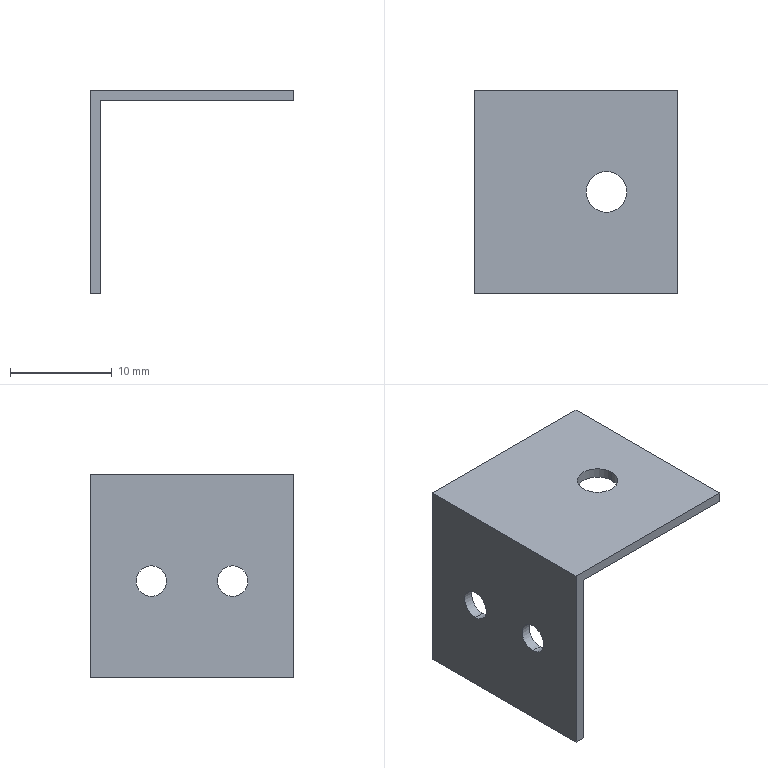Part | SolidWorks | features BaseBody 1 | 1 solid | 14 faces | box 20 x 20 x 20 mm | volume 753.296 mm3 | plane 8 | cylinder 6 | commonest cylinder face diameters 3 x4 4 x2
STEP:
#1=CARTESIAN_POINT('',(1.,10.,10.));
#2=VERTEX_POINT('',#1);
#3=CARTESIAN_POINT('',(5.,10.,10.));
#4=VERTEX_POINT('',#3);
#5=CARTESIAN_POINT('',(3.,10.,10.));
#6=DIRECTION('',(0.,0.,1.));
#7=DIRECTION('',(-1.,0.,0.));
#8=AXIS2_PLACEMENT_3D('',#5,#6,#7);
#9=CIRCLE('',#8,2.);
#10=EDGE_CURVE('',#2,#4,#9,.T.);
#11=ORIENTED_EDGE('',*,*,#10,.T.);
#12=CARTESIAN_POINT('',(5.,10.,9.));
#13=VERTEX_POINT('',#12);
#14=CARTESIAN_POINT('',(5.,10.,10.));
#15=DIRECTION('',(0.,0.,-1.));
#16=VECTOR('',#15,1000.);
#17=LINE('',#14,#16);
#18=EDGE_CURVE('',#4,#13,#17,.T.);
#19=ORIENTED_EDGE('',*,*,#18,.T.);
#20=CARTESIAN_POINT('',(1.,10.,9.));
#21=VERTEX_POINT('',#20);
#22=CARTESIAN_POINT('',(3.,10.,9.));
#23=DIRECTION('',(0.,0.,1.));
#24=DIRECTION('',(-1.,0.,0.));
#25=AXIS2_PLACEMENT_3D('',#22,#23,#24);
#26=CIRCLE('',#25,2.);
#27=EDGE_CURVE('',#21,#13,#26,.T.);
#28=ORIENTED_EDGE('',*,*,#27,.F.);
#29=CARTESIAN_POINT('',(1.,10.,10.));
#30=DIRECTION('',(0.,0.,-1.));
#31=VECTOR('',#30,1000.);
#32=LINE('',#29,#31);
#33=EDGE_CURVE('',#2,#21,#32,.T.);
#34=ORIENTED_EDGE('',*,*,#33,.F.);
#35=EDGE_LOOP('',(#11,#19,#28,#34));
#36=FACE_OUTER_BOUND('',#35,.T.);
#37=CARTESIAN_POINT('',(3.,10.,10.));
#38=DIRECTION('',(0.,0.,-1.));
#39=DIRECTION('',(-1.,0.,0.));
#40=AXIS2_PLACEMENT_3D('',#37,#38,#39);
#41=CYLINDRICAL_SURFACE('',#40,2.);
#42=ADVANCED_FACE('',(#36),#41,.F.);
#43=CARTESIAN_POINT('',(-10.,6.,1.));
#44=VERTEX_POINT('',#43);
#45=CARTESIAN_POINT('',(-10.,6.,-2.));
#46=VERTEX_POINT('',#45);
#47=CARTESIAN_POINT('',(-10.,6.,-0.5));
#48=DIRECTION('',(1.,0.,0.));
#49=DIRECTION('',(0.,0.,-1.));
#50=AXIS2_PLACEMENT_3D('',#47,#48,#49);
#51=CIRCLE('',#50,1.5);
#52=EDGE_CURVE('',#44,#46,#51,.T.);
#53=ORIENTED_EDGE('',*,*,#52,.F.);
#54=CARTESIAN_POINT('',(-9.,6.,1.));
#55=VERTEX_POINT('',#54);
#56=CARTESIAN_POINT('',(-29.,6.,1.));
#57=DIRECTION('',(1.,0.,0.));
#58=VECTOR('',#57,1000.);
#59=LINE('',#56,#58);
#60=EDGE_CURVE('',#44,#55,#59,.T.);
#61=ORIENTED_EDGE('',*,*,#60,.T.);
#62=CARTESIAN_POINT('',(-9.,6.,-2.));
#63=VERTEX_POINT('',#62);
#64=CARTESIAN_POINT('',(-9.,6.,-0.5));
#65=DIRECTION('',(-1.,0.,0.));
#66=DIRECTION('',(0.,0.,-1.));
#67=AXIS2_PLACEMENT_3D('',#64,#65,#66);
#68=CIRCLE('',#67,1.5);
#69=EDGE_CURVE('',#63,#55,#68,.T.);
#70=ORIENTED_EDGE('',*,*,#69,.F.);
#71=CARTESIAN_POINT('',(-29.,6.,-2.));
#72=DIRECTION('',(1.,0.,0.));
#73=VECTOR('',#72,1000.);
#74=LINE('',#71,#73);
#75=EDGE_CURVE('',#46,#63,#74,.T.);
#76=ORIENTED_EDGE('',*,*,#75,.F.);
#77=EDGE_LOOP('',(#53,#61,#70,#76));
#78=FACE_OUTER_BOUND('',#77,.T.);
#79=CARTESIAN_POINT('',(-29.,6.,-0.5));
#80=DIRECTION('',(1.,0.,0.));
#81=DIRECTION('',(0.,0.,-1.));
#82=AXIS2_PLACEMENT_3D('',#79,#80,#81);
#83=CYLINDRICAL_SURFACE('',#82,1.5);
#84=ADVANCED_FACE('',(#78),#83,.F.);
#85=CARTESIAN_POINT('',(-10.,14.,1.));
#86=VERTEX_POINT('',#85);
#87=CARTESIAN_POINT('',(-10.,14.,-2.));
#88=VERTEX_POINT('',#87);
#89=CARTESIAN_POINT('',(-10.,14.,-0.5));
#90=DIRECTION('',(1.,0.,0.));
#91=DIRECTION('',(0.,0.,-1.));
#92=AXIS2_PLACEMENT_3D('',#89,#90,#91);
#93=CIRCLE('',#92,1.5);
#94=EDGE_CURVE('',#86,#88,#93,.T.);
#95=ORIENTED_EDGE('',*,*,#94,.F.);
#96=CARTESIAN_POINT('',(-9.,14.,1.));
#97=VERTEX_POINT('',#96);
#98=CARTESIAN_POINT('',(-29.,14.,1.));
#99=DIRECTION('',(1.,0.,0.));
#100=VECTOR('',#99,1000.);
#101=LINE('',#98,#100);
#102=EDGE_CURVE('',#86,#97,#101,.T.);
#103=ORIENTED_EDGE('',*,*,#102,.T.);
#104=CARTESIAN_POINT('',(-9.,14.,-2.));
#105=VERTEX_POINT('',#104);
#106=CARTESIAN_POINT('',(-9.,14.,-0.5));
#107=DIRECTION('',(-1.,0.,0.));
#108=DIRECTION('',(0.,0.,-1.));
#109=AXIS2_PLACEMENT_3D('',#106,#107,#108);
#110=CIRCLE('',#109,1.5);
#111=EDGE_CURVE('',#105,#97,#110,.T.);
#112=ORIENTED_EDGE('',*,*,#111,.F.);
#113=CARTESIAN_POINT('',(-29.,14.,-2.));
#114=DIRECTION('',(1.,0.,0.));
#115=VECTOR('',#114,1000.);
#116=LINE('',#113,#115);
#117=EDGE_CURVE('',#88,#105,#116,.T.);
#118=ORIENTED_EDGE('',*,*,#117,.F.);
#119=EDGE_LOOP('',(#95,#103,#112,#118));
#120=FACE_OUTER_BOUND('',#119,.T.);
#121=CARTESIAN_POINT('',(-29.,14.,-0.5));
#122=DIRECTION('',(1.,0.,0.));
#123=DIRECTION('',(0.,0.,-1.));
#124=AXIS2_PLACEMENT_3D('',#121,#122,#123);
#125=CYLINDRICAL_SURFACE('',#124,1.5);
#126=ADVANCED_FACE('',(#120),#125,.F.);
#127=CARTESIAN_POINT('',(10.,20.,10.));
#128=VERTEX_POINT('',#127);
#129=CARTESIAN_POINT('',(10.,0.,10.));
#130=VERTEX_POINT('',#129);
#131=CARTESIAN_POINT('',(10.,20.,10.));
#132=DIRECTION('',(0.,-1.,0.));
#133=VECTOR('',#132,1000.);
#134=LINE('',#131,#133);
#135=EDGE_CURVE('',#128,#130,#134,.T.);
#136=ORIENTED_EDGE('',*,*,#135,.F.);
#137=CARTESIAN_POINT('',(-10.,20.,10.));
#138=VERTEX_POINT('',#137);
#139=CARTESIAN_POINT('',(0.,20.,10.));
#140=DIRECTION('',(1.,0.,0.));
#141=VECTOR('',#140,1000.);
#142=LINE('',#139,#141);
#143=EDGE_CURVE('',#138,#128,#142,.T.);
#144=ORIENTED_EDGE('',*,*,#143,.F.);
#145=CARTESIAN_POINT('',(-10.,0.,10.));
#146=VERTEX_POINT('',#145);
#147=CARTESIAN_POINT('',(-10.,20.,10.));
#148=DIRECTION('',(0.,1.,0.));
#149=VECTOR('',#148,1000.);
#150=LINE('',#147,#149);
#151=EDGE_CURVE('',#146,#138,#150,.T.);
#152=ORIENTED_EDGE('',*,*,#151,.F.);
#153=CARTESIAN_POINT('',(0.,0.,10.));
#154=DIRECTION('',(-1.,0.,0.));
#155=VECTOR('',#154,1000.);
#156=LINE('',#153,#155);
#157=EDGE_CURVE('',#130,#146,#156,.T.);
#158=ORIENTED_EDGE('',*,*,#157,.F.);
#159=EDGE_LOOP('',(#136,#144,#152,#158));
#160=FACE_OUTER_BOUND('',#159,.T.);
#161=ORIENTED_EDGE('',*,*,#10,.F.);
#162=CARTESIAN_POINT('',(3.,10.,10.));
#163=DIRECTION('',(0.,0.,1.));
#164=DIRECTION('',(-1.,0.,0.));
#165=AXIS2_PLACEMENT_3D('',#162,#163,#164);
#166=CIRCLE('',#165,2.);
#167=EDGE_CURVE('',#4,#2,#166,.T.);
#168=ORIENTED_EDGE('',*,*,#167,.F.);
#169=EDGE_LOOP('',(#161,#168));
#170=FACE_BOUND('',#169,.T.);
#171=CARTESIAN_POINT('',(0.,20.,10.));
#172=DIRECTION('',(0.,0.,-1.));
#173=DIRECTION('',(-1.,0.,0.));
#174=AXIS2_PLACEMENT_3D('',#171,#172,#173);
#175=PLANE('',#174);
#176=ADVANCED_FACE('',(#160,#170),#175,.F.);
#177=CARTESIAN_POINT('',(10.,0.,9.));
#178=VERTEX_POINT('',#177);
#179=CARTESIAN_POINT('',(-9.,0.,9.));
#180=VERTEX_POINT('',#179);
#181=CARTESIAN_POINT('',(0.,0.,9.));
#182=DIRECTION('',(-1.,0.,0.));
#183=VECTOR('',#182,1000.);
#184=LINE('',#181,#183);
#185=EDGE_CURVE('',#178,#180,#184,.T.);
#186=ORIENTED_EDGE('',*,*,#185,.F.);
#187=CARTESIAN_POINT('',(10.,0.,0.));
#188=DIRECTION('',(0.,0.,-1.));
#189=VECTOR('',#188,1000.);
#190=LINE('',#187,#189);
#191=EDGE_CURVE('',#130,#178,#190,.T.);
#192=ORIENTED_EDGE('',*,*,#191,.F.);
#193=ORIENTED_EDGE('',*,*,#157,.T.);
#194=CARTESIAN_POINT('',(-10.,0.,-10.));
#195=VERTEX_POINT('',#194);
#196=CARTESIAN_POINT('',(-10.,0.,0.));
#197=DIRECTION('',(0.,0.,1.));
#198=VECTOR('',#197,1000.);
#199=LINE('',#196,#198);
#200=EDGE_CURVE('',#195,#146,#199,.T.);
#201=ORIENTED_EDGE('',*,*,#200,.F.);
#202=CARTESIAN_POINT('',(-9.,0.,-10.));
#203=VERTEX_POINT('',#202);
#204=CARTESIAN_POINT('',(0.,0.,-10.));
#205=DIRECTION('',(-1.,0.,0.));
#206=VECTOR('',#205,1000.);
#207=LINE('',#204,#206);
#208=EDGE_CURVE('',#203,#195,#207,.T.);
#209=ORIENTED_EDGE('',*,*,#208,.F.);
#210=CARTESIAN_POINT('',(-9.,0.,0.));
#211=DIRECTION('',(0.,0.,-1.));
#212=VECTOR('',#211,1000.);
#213=LINE('',#210,#212);
#214=EDGE_CURVE('',#180,#203,#213,.T.);
#215=ORIENTED_EDGE('',*,*,#214,.F.);
#216=EDGE_LOOP('',(#186,#192,#193,#201,#209,#215));
#217=FACE_OUTER_BOUND('',#216,.T.);
#218=CARTESIAN_POINT('',(0.,0.,0.));
#219=DIRECTION('',(0.,1.,0.));
#220=DIRECTION('',(0.,0.,1.));
#221=AXIS2_PLACEMENT_3D('',#218,#219,#220);
#222=PLANE('',#221);
#223=ADVANCED_FACE('',(#217),#222,.F.);
#224=CARTESIAN_POINT('',(10.,20.,9.));
#225=VERTEX_POINT('',#224);
#226=CARTESIAN_POINT('',(10.,20.,9.));
#227=DIRECTION('',(0.,-1.,0.));
#228=VECTOR('',#227,1000.);
#229=LINE('',#226,#228);
#230=EDGE_CURVE('',#225,#178,#229,.T.);
#231=ORIENTED_EDGE('',*,*,#230,.F.);
#232=CARTESIAN_POINT('',(10.,20.,0.));
#233=DIRECTION('',(0.,0.,-1.));
#234=VECTOR('',#233,1000.);
#235=LINE('',#232,#234);
#236=EDGE_CURVE('',#128,#225,#235,.T.);
#237=ORIENTED_EDGE('',*,*,#236,.F.);
#238=ORIENTED_EDGE('',*,*,#135,.T.);
#239=ORIENTED_EDGE('',*,*,#191,.T.);
#240=EDGE_LOOP('',(#231,#237,#238,#239));
#241=FACE_OUTER_BOUND('',#240,.T.);
#242=CARTESIAN_POINT('',(10.,20.,0.));
#243=DIRECTION('',(-1.,0.,0.));
#244=DIRECTION('',(0.,0.,1.));
#245=AXIS2_PLACEMENT_3D('',#242,#243,#244);
#246=PLANE('',#245);
#247=ADVANCED_FACE('',(#241),#246,.F.);
#248=ORIENTED_EDGE('',*,*,#236,.T.);
#249=CARTESIAN_POINT('',(-9.,20.,9.));
#250=VERTEX_POINT('',#249);
#251=CARTESIAN_POINT('',(0.,20.,9.));
#252=DIRECTION('',(-1.,0.,0.));
#253=VECTOR('',#252,1000.);
#254=LINE('',#251,#253);
#255=EDGE_CURVE('',#225,#250,#254,.T.);
#256=ORIENTED_EDGE('',*,*,#255,.T.);
#257=CARTESIAN_POINT('',(-9.,20.,-10.));
#258=VERTEX_POINT('',#257);
#259=CARTESIAN_POINT('',(-9.,20.,0.));
#260=DIRECTION('',(0.,0.,-1.));
#261=VECTOR('',#260,1000.);
#262=LINE('',#259,#261);
#263=EDGE_CURVE('',#250,#258,#262,.T.);
#264=ORIENTED_EDGE('',*,*,#263,.T.);
#265=CARTESIAN_POINT('',(-10.,20.,-10.));
#266=VERTEX_POINT('',#265);
#267=CARTESIAN_POINT('',(0.,20.,-10.));
#268=DIRECTION('',(1.,0.,0.));
#269=VECTOR('',#268,1000.);
#270=LINE('',#267,#269);
#271=EDGE_CURVE('',#266,#258,#270,.T.);
#272=ORIENTED_EDGE('',*,*,#271,.F.);
#273=CARTESIAN_POINT('',(-10.,20.,0.));
#274=DIRECTION('',(0.,0.,1.));
#275=VECTOR('',#274,1000.);
#276=LINE('',#273,#275);
#277=EDGE_CURVE('',#266,#138,#276,.T.);
#278=ORIENTED_EDGE('',*,*,#277,.T.);
#279=ORIENTED_EDGE('',*,*,#143,.T.);
#280=EDGE_LOOP('',(#248,#256,#264,#272,#278,#279));
#281=FACE_OUTER_BOUND('',#280,.T.);
#282=CARTESIAN_POINT('',(0.,20.,0.));
#283=DIRECTION('',(0.,1.,0.));
#284=DIRECTION('',(0.,0.,1.));
#285=AXIS2_PLACEMENT_3D('',#282,#283,#284);
#286=PLANE('',#285);
#287=ADVANCED_FACE('',(#281),#286,.T.);
#288=ORIENTED_EDGE('',*,*,#277,.F.);
#289=CARTESIAN_POINT('',(-10.,20.,-10.));
#290=DIRECTION('',(0.,-1.,0.));
#291=VECTOR('',#290,1000.);
#292=LINE('',#289,#291);
#293=EDGE_CURVE('',#266,#195,#292,.T.);
#294=ORIENTED_EDGE('',*,*,#293,.T.);
#295=ORIENTED_EDGE('',*,*,#200,.T.);
#296=ORIENTED_EDGE('',*,*,#151,.T.);
#297=EDGE_LOOP('',(#288,#294,#295,#296));
#298=FACE_OUTER_BOUND('',#297,.T.);
#299=CARTESIAN_POINT('',(-10.,6.,-0.5));
#300=DIRECTION('',(1.,0.,0.));
#301=DIRECTION('',(0.,0.,-1.));
#302=AXIS2_PLACEMENT_3D('',#299,#300,#301);
#303=CIRCLE('',#302,1.5);
#304=EDGE_CURVE('',#46,#44,#303,.T.);
#305=ORIENTED_EDGE('',*,*,#304,.T.);
#306=ORIENTED_EDGE('',*,*,#52,.T.);
#307=EDGE_LOOP('',(#305,#306));
#308=FACE_BOUND('',#307,.T.);
#309=CARTESIAN_POINT('',(-10.,14.,-0.5));
#310=DIRECTION('',(1.,0.,0.));
#311=DIRECTION('',(0.,0.,-1.));
#312=AXIS2_PLACEMENT_3D('',#309,#310,#311);
#313=CIRCLE('',#312,1.5);
#314=EDGE_CURVE('',#88,#86,#313,.T.);
#315=ORIENTED_EDGE('',*,*,#314,.T.);
#316=ORIENTED_EDGE('',*,*,#94,.T.);
#317=EDGE_LOOP('',(#315,#316));
#318=FACE_BOUND('',#317,.T.);
#319=CARTESIAN_POINT('',(-10.,20.,0.));
#320=DIRECTION('',(-1.,0.,0.));
#321=DIRECTION('',(0.,0.,1.));
#322=AXIS2_PLACEMENT_3D('',#319,#320,#321);
#323=PLANE('',#322);
#324=ADVANCED_FACE('',(#298,#308,#318),#323,.T.);
#325=ORIENTED_EDGE('',*,*,#18,.F.);
#326=ORIENTED_EDGE('',*,*,#167,.T.);
#327=ORIENTED_EDGE('',*,*,#33,.T.);
#328=CARTESIAN_POINT('',(3.,10.,9.));
#329=DIRECTION('',(0.,0.,1.));
#330=DIRECTION('',(-1.,0.,0.));
#331=AXIS2_PLACEMENT_3D('',#328,#329,#330);
#332=CIRCLE('',#331,2.);
#333=EDGE_CURVE('',#13,#21,#332,.T.);
#334=ORIENTED_EDGE('',*,*,#333,.F.);
#335=EDGE_LOOP('',(#325,#326,#327,#334));
#336=FACE_OUTER_BOUND('',#335,.T.);
#337=CARTESIAN_POINT('',(3.,10.,10.));
#338=DIRECTION('',(0.,0.,-1.));
#339=DIRECTION('',(-1.,0.,0.));
#340=AXIS2_PLACEMENT_3D('',#337,#338,#339);
#341=CYLINDRICAL_SURFACE('',#340,2.);
#342=ADVANCED_FACE('',(#336),#341,.F.);
#343=ORIENTED_EDGE('',*,*,#263,.F.);
#344=CARTESIAN_POINT('',(-9.,20.,9.));
#345=DIRECTION('',(0.,-1.,0.));
#346=VECTOR('',#345,1000.);
#347=LINE('',#344,#346);
#348=EDGE_CURVE('',#250,#180,#347,.T.);
#349=ORIENTED_EDGE('',*,*,#348,.T.);
#350=ORIENTED_EDGE('',*,*,#214,.T.);
#351=CARTESIAN_POINT('',(-9.,20.,-10.));
#352=DIRECTION('',(0.,1.,0.));
#353=VECTOR('',#352,1000.);
#354=LINE('',#351,#353);
#355=EDGE_CURVE('',#203,#258,#354,.T.);
#356=ORIENTED_EDGE('',*,*,#355,.T.);
#357=EDGE_LOOP('',(#343,#349,#350,#356));
#358=FACE_OUTER_BOUND('',#357,.T.);
#359=ORIENTED_EDGE('',*,*,#69,.T.);
#360=CARTESIAN_POINT('',(-9.,6.,-0.5));
#361=DIRECTION('',(-1.,0.,0.));
#362=DIRECTION('',(0.,0.,-1.));
#363=AXIS2_PLACEMENT_3D('',#360,#361,#362);
#364=CIRCLE('',#363,1.5);
#365=EDGE_CURVE('',#55,#63,#364,.T.);
#366=ORIENTED_EDGE('',*,*,#365,.T.);
#367=EDGE_LOOP('',(#359,#366));
#368=FACE_BOUND('',#367,.T.);
#369=ORIENTED_EDGE('',*,*,#111,.T.);
#370=CARTESIAN_POINT('',(-9.,14.,-0.5));
#371=DIRECTION('',(-1.,0.,0.));
#372=DIRECTION('',(0.,0.,-1.));
#373=AXIS2_PLACEMENT_3D('',#370,#371,#372);
#374=CIRCLE('',#373,1.5);
#375=EDGE_CURVE('',#97,#105,#374,.T.);
#376=ORIENTED_EDGE('',*,*,#375,.T.);
#377=EDGE_LOOP('',(#369,#376));
#378=FACE_BOUND('',#377,.T.);
#379=CARTESIAN_POINT('',(-9.,20.,0.));
#380=DIRECTION('',(1.,0.,0.));
#381=DIRECTION('',(0.,0.,-1.));
#382=AXIS2_PLACEMENT_3D('',#379,#380,#381);
#383=PLANE('',#382);
#384=ADVANCED_FACE('',(#358,#368,#378),#383,.T.);
#385=ORIENTED_EDGE('',*,*,#348,.F.);
#386=ORIENTED_EDGE('',*,*,#255,.F.);
#387=ORIENTED_EDGE('',*,*,#230,.T.);
#388=ORIENTED_EDGE('',*,*,#185,.T.);
#389=EDGE_LOOP('',(#385,#386,#387,#388));
#390=FACE_OUTER_BOUND('',#389,.T.);
#391=ORIENTED_EDGE('',*,*,#27,.T.);
#392=ORIENTED_EDGE('',*,*,#333,.T.);
#393=EDGE_LOOP('',(#391,#392));
#394=FACE_BOUND('',#393,.T.);
#395=CARTESIAN_POINT('',(0.,20.,9.));
#396=DIRECTION('',(0.,0.,1.));
#397=DIRECTION('',(1.,0.,0.));
#398=AXIS2_PLACEMENT_3D('',#395,#396,#397);
#399=PLANE('',#398);
#400=ADVANCED_FACE('',(#390,#394),#399,.F.);
#401=ORIENTED_EDGE('',*,*,#271,.T.);
#402=ORIENTED_EDGE('',*,*,#355,.F.);
#403=ORIENTED_EDGE('',*,*,#208,.T.);
#404=ORIENTED_EDGE('',*,*,#293,.F.);
#405=EDGE_LOOP('',(#401,#402,#403,#404));
#406=FACE_OUTER_BOUND('',#405,.T.);
#407=CARTESIAN_POINT('',(0.,20.,-10.));
#408=DIRECTION('',(0.,0.,-1.));
#409=DIRECTION('',(-1.,0.,0.));
#410=AXIS2_PLACEMENT_3D('',#407,#408,#409);
#411=PLANE('',#410);
#412=ADVANCED_FACE('',(#406),#411,.T.);
#413=ORIENTED_EDGE('',*,*,#60,.F.);
#414=ORIENTED_EDGE('',*,*,#304,.F.);
#415=ORIENTED_EDGE('',*,*,#75,.T.);
#416=ORIENTED_EDGE('',*,*,#365,.F.);
#417=EDGE_LOOP('',(#413,#414,#415,#416));
#418=FACE_OUTER_BOUND('',#417,.T.);
#419=CARTESIAN_POINT('',(-29.,6.,-0.5));
#420=DIRECTION('',(1.,0.,0.));
#421=DIRECTION('',(0.,0.,-1.));
#422=AXIS2_PLACEMENT_3D('',#419,#420,#421);
#423=CYLINDRICAL_SURFACE('',#422,1.5);
#424=ADVANCED_FACE('',(#418),#423,.F.);
#425=ORIENTED_EDGE('',*,*,#102,.F.);
#426=ORIENTED_EDGE('',*,*,#314,.F.);
#427=ORIENTED_EDGE('',*,*,#117,.T.);
#428=ORIENTED_EDGE('',*,*,#375,.F.);
#429=EDGE_LOOP('',(#425,#426,#427,#428));
#430=FACE_OUTER_BOUND('',#429,.T.);
#431=CARTESIAN_POINT('',(-29.,14.,-0.5));
#432=DIRECTION('',(1.,0.,0.));
#433=DIRECTION('',(0.,0.,-1.));
#434=AXIS2_PLACEMENT_3D('',#431,#432,#433);
#435=CYLINDRICAL_SURFACE('',#434,1.5);
#436=ADVANCED_FACE('',(#430),#435,.F.);
#437=CLOSED_SHELL('',(#42,#84,#126,#176,#223,#247,#287,#324,#342,#384,#400,#412,#424,#436));
#438=MANIFOLD_SOLID_BREP('',#437);
#439=CARTESIAN_POINT('',(0.,0.,0.));
#440=DIRECTION('',(0.,0.,1.));
#441=DIRECTION('',(1.,0.,0.));
#442=AXIS2_PLACEMENT_3D('',#439,#440,#441);
#443=(LENGTH_UNIT()NAMED_UNIT(*)SI_UNIT(.MILLI.,.METRE.));
#444=UNCERTAINTY_MEASURE_WITH_UNIT(LENGTH_MEASURE(0.00001),#443,'','');
#445=(NAMED_UNIT(*)PLANE_ANGLE_UNIT()SI_UNIT($,.RADIAN.));
#446=(NAMED_UNIT(*)SI_UNIT($,.STERADIAN.)SOLID_ANGLE_UNIT());
#447=(GEOMETRIC_REPRESENTATION_CONTEXT(3)GLOBAL_UNCERTAINTY_ASSIGNED_CONTEXT((#444))GLOBAL_UNIT_ASSIGNED_CONTEXT((#443,#445,#446))REPRESENTATION_CONTEXT('',''));
#448=ADVANCED_BREP_SHAPE_REPRESENTATION('',(#438,#442),#447);